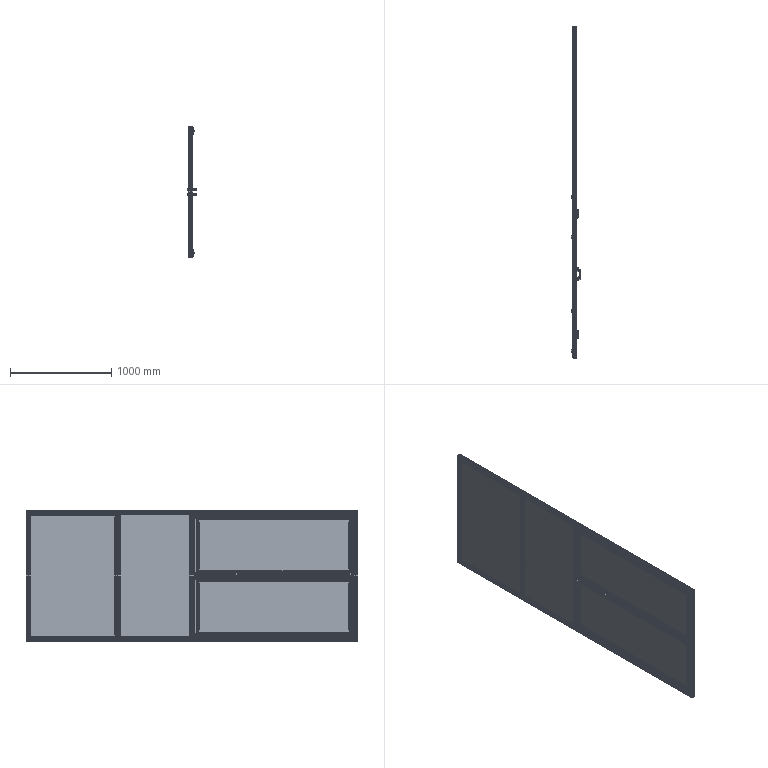Part | SolidWorks | 128 solids | 6042 faces | volume 29490939 mm3 | plane 3794 | cylinder 1852 | cone 372 | spline 24 | commonest cylinder face diameters 6.8 x258 2 x180 5 x148 1.5 x96 19 x96 20.854 x96